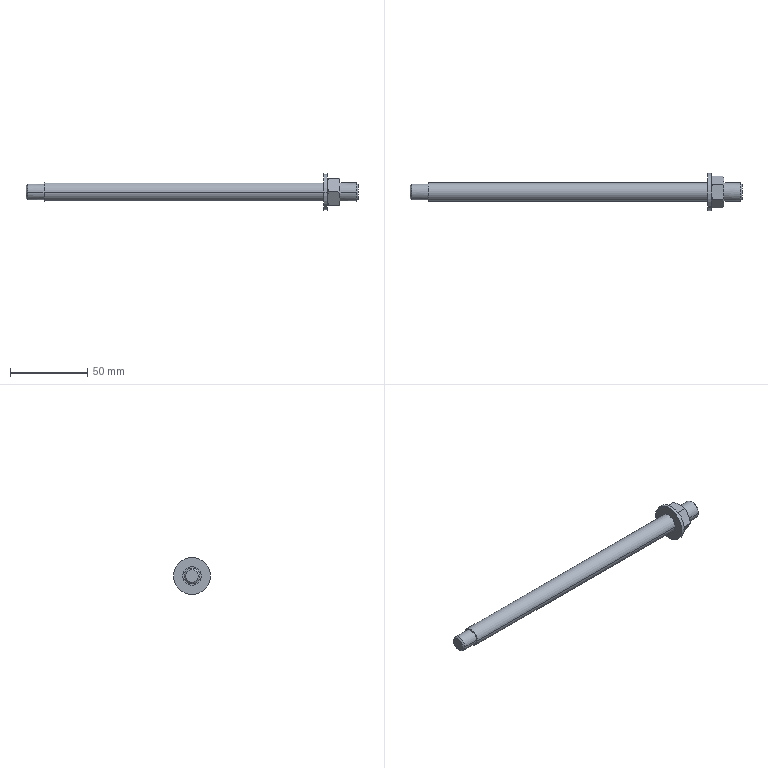Part | NX | features BREP 1 | 1 solid | 36 faces | box 215 x 24 x 24 mm | volume 26001 mm3 | cone 16 | plane 12 | cylinder 8 | commonest cylinder face diameters 12 x4 10.2 x2 24 x2
STEP:
#1=CARTESIAN_POINT('',(0.,-6.,0.));
#2=VERTEX_POINT('',#1);
#3=CARTESIAN_POINT('',(0.,6.,0.));
#4=VERTEX_POINT('',#3);
#5=CARTESIAN_POINT('',(0.,0.,0.));
#6=DIRECTION('',(-1.,0.,0.));
#7=DIRECTION('',(0.,-1.,0.));
#8=AXIS2_PLACEMENT_3D('',#5,#6,#7);
#9=CIRCLE('',#8,6.);
#10=EDGE_CURVE('',#2,#4,#9,.T.);
#11=ORIENTED_EDGE('',*,*,#10,.T.);
#12=CARTESIAN_POINT('',(-181.107,6.,0.));
#13=VERTEX_POINT('',#12);
#14=CARTESIAN_POINT('',(-192.773,6.,0.));
#15=DIRECTION('',(-1.,0.,0.));
#16=VECTOR('',#15,1000.);
#17=LINE('',#14,#16);
#18=EDGE_CURVE('',#4,#13,#17,.T.);
#19=ORIENTED_EDGE('',*,*,#18,.T.);
#20=CARTESIAN_POINT('',(-181.107,-6.,0.));
#21=VERTEX_POINT('',#20);
#22=CARTESIAN_POINT('',(-181.107,0.,0.));
#23=DIRECTION('',(1.,0.,0.));
#24=DIRECTION('',(0.,-1.,0.));
#25=AXIS2_PLACEMENT_3D('',#22,#23,#24);
#26=CIRCLE('',#25,6.);
#27=EDGE_CURVE('',#13,#21,#26,.T.);
#28=ORIENTED_EDGE('',*,*,#27,.T.);
#29=CARTESIAN_POINT('',(-192.773,-6.,0.));
#30=DIRECTION('',(-1.,0.,0.));
#31=VECTOR('',#30,1000.);
#32=LINE('',#29,#31);
#33=EDGE_CURVE('',#2,#21,#32,.T.);
#34=ORIENTED_EDGE('',*,*,#33,.F.);
#35=EDGE_LOOP('',(#11,#19,#28,#34));
#36=FACE_BOUND('',#35,.T.);
#37=CARTESIAN_POINT('',(-192.773,0.,0.));
#38=DIRECTION('',(-1.,0.,0.));
#39=DIRECTION('',(0.,-1.,0.));
#40=AXIS2_PLACEMENT_3D('',#37,#38,#39);
#41=CYLINDRICAL_SURFACE('',#40,6.);
#42=ADVANCED_FACE('',(#36),#41,.T.);
#43=CARTESIAN_POINT('',(-181.107,-5.1,0.));
#44=VERTEX_POINT('',#43);
#45=CARTESIAN_POINT('',(-181.107,5.1,0.));
#46=VERTEX_POINT('',#45);
#47=CARTESIAN_POINT('',(-181.107,0.,0.));
#48=DIRECTION('',(-1.,0.,0.));
#49=DIRECTION('',(0.,-1.,0.));
#50=AXIS2_PLACEMENT_3D('',#47,#48,#49);
#51=CIRCLE('',#50,5.1);
#52=EDGE_CURVE('',#44,#46,#51,.T.);
#53=ORIENTED_EDGE('',*,*,#52,.T.);
#54=CARTESIAN_POINT('',(-191.753,5.1,0.));
#55=VERTEX_POINT('',#54);
#56=CARTESIAN_POINT('',(-192.773,5.1,0.));
#57=DIRECTION('',(-1.,0.,0.));
#58=VECTOR('',#57,1000.);
#59=LINE('',#56,#58);
#60=EDGE_CURVE('',#46,#55,#59,.T.);
#61=ORIENTED_EDGE('',*,*,#60,.T.);
#62=CARTESIAN_POINT('',(-191.753,0.,5.1));
#63=VERTEX_POINT('',#62);
#64=CARTESIAN_POINT('',(-191.753,0.,0.));
#65=DIRECTION('',(1.,0.,0.));
#66=DIRECTION('',(0.,-1.,0.));
#67=AXIS2_PLACEMENT_3D('',#64,#65,#66);
#68=CIRCLE('',#67,5.1);
#69=EDGE_CURVE('',#55,#63,#68,.T.);
#70=ORIENTED_EDGE('',*,*,#69,.T.);
#71=CARTESIAN_POINT('',(-191.753,-5.1,0.));
#72=VERTEX_POINT('',#71);
#73=CARTESIAN_POINT('',(-191.753,0.,0.));
#74=DIRECTION('',(1.,0.,0.));
#75=DIRECTION('',(0.,-1.,0.));
#76=AXIS2_PLACEMENT_3D('',#73,#74,#75);
#77=CIRCLE('',#76,5.1);
#78=EDGE_CURVE('',#63,#72,#77,.T.);
#79=ORIENTED_EDGE('',*,*,#78,.T.);
#80=CARTESIAN_POINT('',(-192.773,-5.1,0.));
#81=DIRECTION('',(-1.,0.,0.));
#82=VECTOR('',#81,1000.);
#83=LINE('',#80,#82);
#84=EDGE_CURVE('',#44,#72,#83,.T.);
#85=ORIENTED_EDGE('',*,*,#84,.F.);
#86=EDGE_LOOP('',(#53,#61,#70,#79,#85));
#87=FACE_BOUND('',#86,.T.);
#88=CARTESIAN_POINT('',(-192.773,0.,0.));
#89=DIRECTION('',(-1.,0.,0.));
#90=DIRECTION('',(0.,-1.,0.));
#91=AXIS2_PLACEMENT_3D('',#88,#89,#90);
#92=CYLINDRICAL_SURFACE('',#91,5.1);
#93=ADVANCED_FACE('',(#87),#92,.T.);
#94=CARTESIAN_POINT('',(2.4,-12.,0.));
#95=VERTEX_POINT('',#94);
#96=CARTESIAN_POINT('',(2.4,12.,0.));
#97=VERTEX_POINT('',#96);
#98=CARTESIAN_POINT('',(2.4,0.,0.));
#99=DIRECTION('',(-1.,0.,0.));
#100=DIRECTION('',(0.,-1.,0.));
#101=AXIS2_PLACEMENT_3D('',#98,#99,#100);
#102=CIRCLE('',#101,12.);
#103=EDGE_CURVE('',#95,#97,#102,.T.);
#104=ORIENTED_EDGE('',*,*,#103,.T.);
#105=CARTESIAN_POINT('',(0.,12.,0.));
#106=VERTEX_POINT('',#105);
#107=CARTESIAN_POINT('',(-192.773,12.,0.));
#108=DIRECTION('',(-1.,0.,0.));
#109=VECTOR('',#108,1000.);
#110=LINE('',#107,#109);
#111=EDGE_CURVE('',#97,#106,#110,.T.);
#112=ORIENTED_EDGE('',*,*,#111,.T.);
#113=CARTESIAN_POINT('',(0.,-12.,0.));
#114=VERTEX_POINT('',#113);
#115=CARTESIAN_POINT('',(0.,0.,0.));
#116=DIRECTION('',(1.,0.,0.));
#117=DIRECTION('',(0.,-1.,0.));
#118=AXIS2_PLACEMENT_3D('',#115,#116,#117);
#119=CIRCLE('',#118,12.);
#120=EDGE_CURVE('',#106,#114,#119,.T.);
#121=ORIENTED_EDGE('',*,*,#120,.T.);
#122=CARTESIAN_POINT('',(-192.773,-12.,0.));
#123=DIRECTION('',(-1.,0.,0.));
#124=VECTOR('',#123,1000.);
#125=LINE('',#122,#124);
#126=EDGE_CURVE('',#95,#114,#125,.T.);
#127=ORIENTED_EDGE('',*,*,#126,.F.);
#128=EDGE_LOOP('',(#104,#112,#121,#127));
#129=FACE_BOUND('',#128,.T.);
#130=CARTESIAN_POINT('',(-192.773,0.,0.));
#131=DIRECTION('',(-1.,0.,0.));
#132=DIRECTION('',(0.,-1.,0.));
#133=AXIS2_PLACEMENT_3D('',#130,#131,#132);
#134=CYLINDRICAL_SURFACE('',#133,12.);
#135=ADVANCED_FACE('',(#129),#134,.T.);
#136=CARTESIAN_POINT('',(-192.773,0.,-4.08));
#137=VERTEX_POINT('',#136);
#138=CARTESIAN_POINT('',(-192.773,0.,4.08));
#139=VERTEX_POINT('',#138);
#140=CARTESIAN_POINT('',(-192.773,0.,0.));
#141=DIRECTION('',(1.,0.,0.));
#142=DIRECTION('',(0.,0.,-1.));
#143=AXIS2_PLACEMENT_3D('',#140,#141,#142);
#144=CIRCLE('',#143,4.08);
#145=EDGE_CURVE('',#137,#139,#144,.T.);
#146=ORIENTED_EDGE('',*,*,#145,.T.);
#147=CARTESIAN_POINT('',(-191.753,0.,5.1));
#148=DIRECTION('',(0.7071,0.,0.7071));
#149=VECTOR('',#148,1000.);
#150=LINE('',#147,#149);
#151=EDGE_CURVE('',#139,#63,#150,.T.);
#152=ORIENTED_EDGE('',*,*,#151,.T.);
#153=ORIENTED_EDGE('',*,*,#69,.F.);
#154=CARTESIAN_POINT('',(-191.753,0.,-5.1));
#155=VERTEX_POINT('',#154);
#156=CARTESIAN_POINT('',(-191.753,0.,0.));
#157=DIRECTION('',(1.,0.,0.));
#158=DIRECTION('',(0.,-1.,0.));
#159=AXIS2_PLACEMENT_3D('',#156,#157,#158);
#160=CIRCLE('',#159,5.1);
#161=EDGE_CURVE('',#155,#55,#160,.T.);
#162=ORIENTED_EDGE('',*,*,#161,.F.);
#163=CARTESIAN_POINT('',(-191.753,0.,-5.1));
#164=DIRECTION('',(0.7071,0.,-0.7071));
#165=VECTOR('',#164,1000.);
#166=LINE('',#163,#165);
#167=EDGE_CURVE('',#137,#155,#166,.T.);
#168=ORIENTED_EDGE('',*,*,#167,.F.);
#169=EDGE_LOOP('',(#146,#152,#153,#162,#168));
#170=FACE_BOUND('',#169,.T.);
#171=CARTESIAN_POINT('',(-191.753,0.,0.));
#172=DIRECTION('',(1.,0.,0.));
#173=DIRECTION('',(0.,0.,-1.));
#174=AXIS2_PLACEMENT_3D('',#171,#172,#173);
#175=CONICAL_SURFACE('',#174,5.1,0.7854);
#176=ADVANCED_FACE('',(#170),#175,.T.);
#177=CARTESIAN_POINT('',(21.207,0.,6.));
#178=VERTEX_POINT('',#177);
#179=CARTESIAN_POINT('',(21.207,6.,0.));
#180=VERTEX_POINT('',#179);
#181=CARTESIAN_POINT('',(21.207,0.,0.));
#182=DIRECTION('',(-1.,0.,0.));
#183=DIRECTION('',(0.,-1.,0.));
#184=AXIS2_PLACEMENT_3D('',#181,#182,#183);
#185=CIRCLE('',#184,6.);
#186=EDGE_CURVE('',#178,#180,#185,.T.);
#187=ORIENTED_EDGE('',*,*,#186,.T.);
#188=CARTESIAN_POINT('',(10.56,6.,0.));
#189=VERTEX_POINT('',#188);
#190=CARTESIAN_POINT('',(-192.773,6.,0.));
#191=DIRECTION('',(-1.,0.,0.));
#192=VECTOR('',#191,1000.);
#193=LINE('',#190,#192);
#194=EDGE_CURVE('',#180,#189,#193,.T.);
#195=ORIENTED_EDGE('',*,*,#194,.T.);
#196=CARTESIAN_POINT('',(10.56,-6.,0.));
#197=VERTEX_POINT('',#196);
#198=CARTESIAN_POINT('',(10.56,0.,0.));
#199=DIRECTION('',(1.,0.,0.));
#200=DIRECTION('',(0.,-1.,0.));
#201=AXIS2_PLACEMENT_3D('',#198,#199,#200);
#202=CIRCLE('',#201,6.);
#203=EDGE_CURVE('',#189,#197,#202,.T.);
#204=ORIENTED_EDGE('',*,*,#203,.T.);
#205=CARTESIAN_POINT('',(21.207,-6.,0.));
#206=VERTEX_POINT('',#205);
#207=CARTESIAN_POINT('',(-192.773,-6.,0.));
#208=DIRECTION('',(-1.,0.,0.));
#209=VECTOR('',#208,1000.);
#210=LINE('',#207,#209);
#211=EDGE_CURVE('',#206,#197,#210,.T.);
#212=ORIENTED_EDGE('',*,*,#211,.F.);
#213=CARTESIAN_POINT('',(21.207,0.,0.));
#214=DIRECTION('',(-1.,0.,0.));
#215=DIRECTION('',(0.,-1.,0.));
#216=AXIS2_PLACEMENT_3D('',#213,#214,#215);
#217=CIRCLE('',#216,6.);
#218=EDGE_CURVE('',#206,#178,#217,.T.);
#219=ORIENTED_EDGE('',*,*,#218,.T.);
#220=EDGE_LOOP('',(#187,#195,#204,#212,#219));
#221=FACE_BOUND('',#220,.T.);
#222=CARTESIAN_POINT('',(-192.773,0.,0.));
#223=DIRECTION('',(-1.,0.,0.));
#224=DIRECTION('',(0.,-1.,0.));
#225=AXIS2_PLACEMENT_3D('',#222,#223,#224);
#226=CYLINDRICAL_SURFACE('',#225,6.);
#227=ADVANCED_FACE('',(#221),#226,.T.);
#228=CARTESIAN_POINT('',(22.227,0.,4.98));
#229=VERTEX_POINT('',#228);
#230=CARTESIAN_POINT('',(22.227,0.,-4.98));
#231=VERTEX_POINT('',#230);
#232=CARTESIAN_POINT('',(22.227,0.,0.));
#233=DIRECTION('',(-1.,0.,0.));
#234=DIRECTION('',(0.,0.,1.));
#235=AXIS2_PLACEMENT_3D('',#232,#233,#234);
#236=CIRCLE('',#235,4.98);
#237=EDGE_CURVE('',#229,#231,#236,.T.);
#238=ORIENTED_EDGE('',*,*,#237,.T.);
#239=CARTESIAN_POINT('',(21.207,0.,-6.));
#240=VERTEX_POINT('',#239);
#241=CARTESIAN_POINT('',(21.207,0.,-6.));
#242=DIRECTION('',(-0.7071,0.,-0.7071));
#243=VECTOR('',#242,1000.);
#244=LINE('',#241,#243);
#245=EDGE_CURVE('',#240,#231,#244,.F.);
#246=ORIENTED_EDGE('',*,*,#245,.F.);
#247=CARTESIAN_POINT('',(21.207,0.,0.));
#248=DIRECTION('',(-1.,0.,0.));
#249=DIRECTION('',(0.,-1.,0.));
#250=AXIS2_PLACEMENT_3D('',#247,#248,#249);
#251=CIRCLE('',#250,6.);
#252=EDGE_CURVE('',#180,#240,#251,.T.);
#253=ORIENTED_EDGE('',*,*,#252,.F.);
#254=ORIENTED_EDGE('',*,*,#186,.F.);
#255=CARTESIAN_POINT('',(21.207,0.,6.));
#256=DIRECTION('',(-0.7071,0.,0.7071));
#257=VECTOR('',#256,1000.);
#258=LINE('',#255,#257);
#259=EDGE_CURVE('',#178,#229,#258,.F.);
#260=ORIENTED_EDGE('',*,*,#259,.T.);
#261=EDGE_LOOP('',(#238,#246,#253,#254,#260));
#262=FACE_BOUND('',#261,.T.);
#263=CARTESIAN_POINT('',(21.207,0.,0.));
#264=DIRECTION('',(-1.,0.,0.));
#265=DIRECTION('',(0.,0.,1.));
#266=AXIS2_PLACEMENT_3D('',#263,#264,#265);
#267=CONICAL_SURFACE('',#266,6.,0.7854);
#268=ADVANCED_FACE('',(#262),#267,.T.);
#269=ORIENTED_EDGE('',*,*,#18,.F.);
#270=CARTESIAN_POINT('',(0.,0.,0.));
#271=DIRECTION('',(-1.,0.,0.));
#272=DIRECTION('',(0.,-1.,0.));
#273=AXIS2_PLACEMENT_3D('',#270,#271,#272);
#274=CIRCLE('',#273,6.);
#275=EDGE_CURVE('',#4,#2,#274,.T.);
#276=ORIENTED_EDGE('',*,*,#275,.T.);
#277=ORIENTED_EDGE('',*,*,#33,.T.);
#278=CARTESIAN_POINT('',(-181.107,0.,0.));
#279=DIRECTION('',(1.,0.,0.));
#280=DIRECTION('',(0.,-1.,0.));
#281=AXIS2_PLACEMENT_3D('',#278,#279,#280);
#282=CIRCLE('',#281,6.);
#283=EDGE_CURVE('',#21,#13,#282,.T.);
#284=ORIENTED_EDGE('',*,*,#283,.T.);
#285=EDGE_LOOP('',(#269,#276,#277,#284));
#286=FACE_BOUND('',#285,.T.);
#287=CARTESIAN_POINT('',(-192.773,0.,0.));
#288=DIRECTION('',(-1.,0.,0.));
#289=DIRECTION('',(0.,-1.,0.));
#290=AXIS2_PLACEMENT_3D('',#287,#288,#289);
#291=CYLINDRICAL_SURFACE('',#290,6.);
#292=ADVANCED_FACE('',(#286),#291,.T.);
#293=ORIENTED_EDGE('',*,*,#283,.F.);
#294=ORIENTED_EDGE('',*,*,#27,.F.);
#295=EDGE_LOOP('',(#293,#294));
#296=FACE_BOUND('',#295,.T.);
#297=ORIENTED_EDGE('',*,*,#52,.F.);
#298=CARTESIAN_POINT('',(-181.107,0.,0.));
#299=DIRECTION('',(-1.,0.,0.));
#300=DIRECTION('',(0.,-1.,0.));
#301=AXIS2_PLACEMENT_3D('',#298,#299,#300);
#302=CIRCLE('',#301,5.1);
#303=EDGE_CURVE('',#46,#44,#302,.T.);
#304=ORIENTED_EDGE('',*,*,#303,.F.);
#305=EDGE_LOOP('',(#297,#304));
#306=FACE_BOUND('',#305,.T.);
#307=CARTESIAN_POINT('',(-181.107,5.1,0.));
#308=DIRECTION('',(1.,0.,0.));
#309=DIRECTION('',(0.,-1.,0.));
#310=AXIS2_PLACEMENT_3D('',#307,#308,#309);
#311=PLANE('',#310);
#312=ADVANCED_FACE('',(#296,#306),#311,.F.);
#313=CARTESIAN_POINT('',(0.,0.,0.));
#314=DIRECTION('',(1.,0.,0.));
#315=DIRECTION('',(0.,-1.,0.));
#316=AXIS2_PLACEMENT_3D('',#313,#314,#315);
#317=CIRCLE('',#316,12.);
#318=EDGE_CURVE('',#114,#106,#317,.T.);
#319=ORIENTED_EDGE('',*,*,#318,.F.);
#320=ORIENTED_EDGE('',*,*,#120,.F.);
#321=EDGE_LOOP('',(#319,#320));
#322=FACE_BOUND('',#321,.T.);
#323=ORIENTED_EDGE('',*,*,#10,.F.);
#324=ORIENTED_EDGE('',*,*,#275,.F.);
#325=EDGE_LOOP('',(#323,#324));
#326=FACE_BOUND('',#325,.T.);
#327=CARTESIAN_POINT('',(0.,6.,0.));
#328=DIRECTION('',(1.,0.,0.));
#329=DIRECTION('',(0.,-1.,0.));
#330=AXIS2_PLACEMENT_3D('',#327,#328,#329);
#331=PLANE('',#330);
#332=ADVANCED_FACE('',(#322,#326),#331,.F.);
#333=ORIENTED_EDGE('',*,*,#60,.F.);
#334=ORIENTED_EDGE('',*,*,#303,.T.);
#335=ORIENTED_EDGE('',*,*,#84,.T.);
#336=CARTESIAN_POINT('',(-191.753,0.,0.));
#337=DIRECTION('',(1.,0.,0.));
#338=DIRECTION('',(0.,-1.,0.));
#339=AXIS2_PLACEMENT_3D('',#336,#337,#338);
#340=CIRCLE('',#339,5.1);
#341=EDGE_CURVE('',#72,#155,#340,.T.);
#342=ORIENTED_EDGE('',*,*,#341,.T.);
#343=ORIENTED_EDGE('',*,*,#161,.T.);
#344=EDGE_LOOP('',(#333,#334,#335,#342,#343));
#345=FACE_BOUND('',#344,.T.);
#346=CARTESIAN_POINT('',(-192.773,0.,0.));
#347=DIRECTION('',(-1.,0.,0.));
#348=DIRECTION('',(0.,-1.,0.));
#349=AXIS2_PLACEMENT_3D('',#346,#347,#348);
#350=CYLINDRICAL_SURFACE('',#349,5.1);
#351=ADVANCED_FACE('',(#345),#350,.T.);
#352=ORIENTED_EDGE('',*,*,#111,.F.);
#353=CARTESIAN_POINT('',(2.4,0.,0.));
#354=DIRECTION('',(-1.,0.,0.));
#355=DIRECTION('',(0.,-1.,0.));
#356=AXIS2_PLACEMENT_3D('',#353,#354,#355);
#357=CIRCLE('',#356,12.);
#358=EDGE_CURVE('',#97,#95,#357,.T.);
#359=ORIENTED_EDGE('',*,*,#358,.T.);
#360=ORIENTED_EDGE('',*,*,#126,.T.);
#361=ORIENTED_EDGE('',*,*,#318,.T.);
#362=EDGE_LOOP('',(#352,#359,#360,#361));
#363=FACE_BOUND('',#362,.T.);
#364=CARTESIAN_POINT('',(-192.773,0.,0.));
#365=DIRECTION('',(-1.,0.,0.));
#366=DIRECTION('',(0.,-1.,0.));
#367=AXIS2_PLACEMENT_3D('',#364,#365,#366);
#368=CYLINDRICAL_SURFACE('',#367,12.);
#369=ADVANCED_FACE('',(#363),#368,.T.);
#370=ORIENTED_EDGE('',*,*,#151,.F.);
#371=CARTESIAN_POINT('',(-192.773,0.,0.));
#372=DIRECTION('',(1.,0.,0.));
#373=DIRECTION('',(0.,0.,-1.));
#374=AXIS2_PLACEMENT_3D('',#371,#372,#373);
#375=CIRCLE('',#374,4.08);
#376=EDGE_CURVE('',#139,#137,#375,.T.);
#377=ORIENTED_EDGE('',*,*,#376,.T.);
#378=ORIENTED_EDGE('',*,*,#167,.T.);
#379=ORIENTED_EDGE('',*,*,#341,.F.);
#380=ORIENTED_EDGE('',*,*,#78,.F.);
#381=EDGE_LOOP('',(#370,#377,#378,#379,#380));
#382=FACE_BOUND('',#381,.T.);
#383=CARTESIAN_POINT('',(-191.753,0.,0.));
#384=DIRECTION('',(1.,0.,0.));
#385=DIRECTION('',(0.,0.,-1.));
#386=AXIS2_PLACEMENT_3D('',#383,#384,#385);
#387=CONICAL_SURFACE('',#386,5.1,0.7854);
#388=ADVANCED_FACE('',(#382),#387,.T.);
#389=ORIENTED_EDGE('',*,*,#103,.F.);
#390=ORIENTED_EDGE('',*,*,#358,.F.);
#391=EDGE_LOOP('',(#389,#390));
#392=FACE_BOUND('',#391,.T.);
#393=CARTESIAN_POINT('',(2.4,7.65,-4.417));
#394=VERTEX_POINT('',#393);
#395=CARTESIAN_POINT('',(2.4,7.65,4.417));
#396=VERTEX_POINT('',#395);
#397=CARTESIAN_POINT('',(2.4,0.,0.));
#398=DIRECTION('',(1.,0.,0.));
#399=DIRECTION('',(0.,0.,-1.));
#400=AXIS2_PLACEMENT_3D('',#397,#398,#399);
#401=CIRCLE('',#400,8.833);
#402=EDGE_CURVE('',#394,#396,#401,.T.);
#403=ORIENTED_EDGE('',*,*,#402,.F.);
#404=CARTESIAN_POINT('',(2.4,0.,-8.833));
#405=VERTEX_POINT('',#404);
#406=CARTESIAN_POINT('',(2.4,0.,0.));
#407=DIRECTION('',(1.,0.,0.));
#408=DIRECTION('',(0.,0.,-1.));
#409=AXIS2_PLACEMENT_3D('',#406,#407,#408);
#410=CIRCLE('',#409,8.833);
#411=EDGE_CURVE('',#405,#394,#410,.T.);
#412=ORIENTED_EDGE('',*,*,#411,.F.);
#413=CARTESIAN_POINT('',(2.4,-7.65,-4.417));
#414=VERTEX_POINT('',#413);
#415=CARTESIAN_POINT('',(2.4,0.,0.));
#416=DIRECTION('',(1.,0.,0.));
#417=DIRECTION('',(0.,0.,-1.));
#418=AXIS2_PLACEMENT_3D('',#415,#416,#417);
#419=CIRCLE('',#418,8.833);
#420=EDGE_CURVE('',#414,#405,#419,.T.);
#421=ORIENTED_EDGE('',*,*,#420,.F.);
#422=CARTESIAN_POINT('',(2.4,-7.65,4.417));
#423=VERTEX_POINT('',#422);
#424=CARTESIAN_POINT('',(2.4,0.,0.));
#425=DIRECTION('',(1.,0.,0.));
#426=DIRECTION('',(0.,0.,-1.));
#427=AXIS2_PLACEMENT_3D('',#424,#425,#426);
#428=CIRCLE('',#427,8.833);
#429=EDGE_CURVE('',#423,#414,#428,.T.);
#430=ORIENTED_EDGE('',*,*,#429,.F.);
#431=CARTESIAN_POINT('',(2.4,0.,8.833));
#432=VERTEX_POINT('',#431);
#433=CARTESIAN_POINT('',(2.4,0.,0.));
#434=DIRECTION('',(1.,0.,0.));
#435=DIRECTION('',(0.,0.,-1.));
#436=AXIS2_PLACEMENT_3D('',#433,#434,#435);
#437=CIRCLE('',#436,8.833);
#438=EDGE_CURVE('',#432,#423,#437,.T.);
#439=ORIENTED_EDGE('',*,*,#438,.F.);
#440=CARTESIAN_POINT('',(2.4,0.,0.));
#441=DIRECTION('',(1.,0.,0.));
#442=DIRECTION('',(0.,0.,-1.));
#443=AXIS2_PLACEMENT_3D('',#440,#441,#442);
#444=CIRCLE('',#443,8.833);
#445=EDGE_CURVE('',#396,#432,#444,.T.);
#446=ORIENTED_EDGE('',*,*,#445,.F.);
#447=EDGE_LOOP('',(#403,#412,#421,#430,#439,#446));
#448=FACE_BOUND('',#447,.T.);
#449=CARTESIAN_POINT('',(2.4,12.,0.));
#450=DIRECTION('',(-1.,0.,0.));
#451=DIRECTION('',(0.,0.,1.));
#452=AXIS2_PLACEMENT_3D('',#449,#450,#451);
#453=PLANE('',#452);
#454=ADVANCED_FACE('',(#392,#448),#453,.F.);
#455=ORIENTED_EDGE('',*,*,#145,.F.);
#456=ORIENTED_EDGE('',*,*,#376,.F.);
#457=EDGE_LOOP('',(#455,#456));
#458=FACE_BOUND('',#457,.T.);
#459=CARTESIAN_POINT('',(-192.773,0.,0.));
#460=DIRECTION('',(1.,0.,0.));
#461=DIRECTION('',(0.,-1.,0.));
#462=AXIS2_PLACEMENT_3D('',#459,#460,#461);
#463=PLANE('',#462);
#464=ADVANCED_FACE('',(#458),#463,.F.);
#465=ORIENTED_EDGE('',*,*,#402,.T.);
#466=CARTESIAN_POINT('',(3.189,10.2,0.));
#467=VERTEX_POINT('',#466);
#468=CARTESIAN_POINT('',(3.189,10.2,0.));
#469=CARTESIAN_POINT('',(2.934,9.758,0.7653));
#470=CARTESIAN_POINT('',(2.559,8.964,2.142));
#471=CARTESIAN_POINT('',(2.4,8.071,3.688));
#472=CARTESIAN_POINT('',(2.4,7.65,4.417));
#473=B_SPLINE_CURVE_WITH_KNOTS('',3,(#468,#469,#470,#471,#472),.UNSPECIFIED.,.F.,.F.,(4,1,4),(0.,0.5,1.),.UNSPECIFIED.);
#474=EDGE_CURVE('',#396,#467,#473,.F.);
#475=ORIENTED_EDGE('',*,*,#474,.T.);
#476=CARTESIAN_POINT('',(2.4,7.65,-4.417));
#477=CARTESIAN_POINT('',(2.4,8.071,-3.688));
#478=CARTESIAN_POINT('',(2.559,8.964,-2.141));
#479=CARTESIAN_POINT('',(2.934,9.758,-0.7656));
#480=CARTESIAN_POINT('',(3.189,10.2,0.));
#481=B_SPLINE_CURVE_WITH_KNOTS('',3,(#476,#477,#478,#479,#480),.UNSPECIFIED.,.F.,.F.,(4,1,4),(0.,0.5,1.),.UNSPECIFIED.);
#482=EDGE_CURVE('',#467,#394,#481,.F.);
#483=ORIENTED_EDGE('',*,*,#482,.T.);
#484=EDGE_LOOP('',(#465,#475,#483));
#485=FACE_BOUND('',#484,.T.);
#486=CARTESIAN_POINT('',(3.194,0.,0.));
#487=DIRECTION('',(1.,0.,0.));
#488=DIRECTION('',(0.,0.,-1.));
#489=AXIS2_PLACEMENT_3D('',#486,#487,#488);
#490=CONICAL_SURFACE('',#489,10.208,1.047);
#491=ADVANCED_FACE('',(#485),#490,.T.);
#492=CARTESIAN_POINT('',(3.189,5.1,-8.833));
#493=VERTEX_POINT('',#492);
#494=CARTESIAN_POINT('',(3.189,5.1,-8.833));
#495=CARTESIAN_POINT('',(2.934,5.542,-8.068));
#496=CARTESIAN_POINT('',(2.559,6.336,-6.692));
#497=CARTESIAN_POINT('',(2.4,7.229,-5.146));
#498=CARTESIAN_POINT('',(2.4,7.65,-4.417));
#499=B_SPLINE_CURVE_WITH_KNOTS('',3,(#494,#495,#496,#497,#498),.UNSPECIFIED.,.F.,.F.,(4,1,4),(0.,0.5,1.),.UNSPECIFIED.);
#500=EDGE_CURVE('',#394,#493,#499,.F.);
#501=ORIENTED_EDGE('',*,*,#500,.T.);
#502=CARTESIAN_POINT('',(2.4,0.,-8.833));
#503=CARTESIAN_POINT('',(2.4,0.8417,-8.833));
#504=CARTESIAN_POINT('',(2.559,2.627,-8.833));
#505=CARTESIAN_POINT('',(2.934,4.216,-8.833));
#506=CARTESIAN_POINT('',(3.189,5.1,-8.833));
#507=B_SPLINE_CURVE_WITH_KNOTS('',3,(#502,#503,#504,#505,#506),.UNSPECIFIED.,.F.,.F.,(4,1,4),(0.,0.5,1.),.UNSPECIFIED.);
#508=EDGE_CURVE('',#493,#405,#507,.F.);
#509=ORIENTED_EDGE('',*,*,#508,.T.);
#510=ORIENTED_EDGE('',*,*,#411,.T.);
#511=EDGE_LOOP('',(#501,#509,#510));
#512=FACE_BOUND('',#511,.T.);
#513=CARTESIAN_POINT('',(3.194,0.,0.));
#514=DIRECTION('',(1.,0.,0.));
#515=DIRECTION('',(0.,0.,-1.));
#516=AXIS2_PLACEMENT_3D('',#513,#514,#515);
#517=CONICAL_SURFACE('',#516,10.208,1.047);
#518=ADVANCED_FACE('',(#512),#517,.T.);
#519=CARTESIAN_POINT('',(3.189,-5.1,-8.833));
#520=VERTEX_POINT('',#519);
#521=CARTESIAN_POINT('',(3.189,-5.1,-8.833));
#522=CARTESIAN_POINT('',(2.934,-4.216,-8.833));
#523=CARTESIAN_POINT('',(2.559,-2.627,-8.833));
#524=CARTESIAN_POINT('',(2.4,-0.8419,-8.833));
#525=CARTESIAN_POINT('',(2.4,0.,-8.833));
#526=B_SPLINE_CURVE_WITH_KNOTS('',3,(#521,#522,#523,#524,#525),.UNSPECIFIED.,.F.,.F.,(4,1,4),(0.,0.5,1.),.UNSPECIFIED.);
#527=EDGE_CURVE('',#405,#520,#526,.F.);
#528=ORIENTED_EDGE('',*,*,#527,.T.);
#529=CARTESIAN_POINT('',(2.4,-7.65,-4.417));
#530=CARTESIAN_POINT('',(2.4,-7.229,-5.146));
#531=CARTESIAN_POINT('',(2.559,-6.336,-6.692));
#532=CARTESIAN_POINT('',(2.934,-5.542,-8.068));
#533=CARTESIAN_POINT('',(3.189,-5.1,-8.833));
#534=B_SPLINE_CURVE_WITH_KNOTS('',3,(#529,#530,#531,#532,#533),.UNSPECIFIED.,.F.,.F.,(4,1,4),(0.,0.5,1.),.UNSPECIFIED.);
#535=EDGE_CURVE('',#520,#414,#534,.F.);
#536=ORIENTED_EDGE('',*,*,#535,.T.);
#537=ORIENTED_EDGE('',*,*,#420,.T.);
#538=EDGE_LOOP('',(#528,#536,#537));
#539=FACE_BOUND('',#538,.T.);
#540=CARTESIAN_POINT('',(3.194,0.,0.));
#541=DIRECTION('',(1.,0.,0.));
#542=DIRECTION('',(0.,0.,-1.));
#543=AXIS2_PLACEMENT_3D('',#540,#541,#542);
#544=CONICAL_SURFACE('',#543,10.208,1.047);
#545=ADVANCED_FACE('',(#539),#544,.T.);
#546=ORIENTED_EDGE('',*,*,#429,.T.);
#547=CARTESIAN_POINT('',(3.189,-10.2,0.000000043));
#548=VERTEX_POINT('',#547);
#549=CARTESIAN_POINT('',(3.189,-10.2,0.000000022));
#550=CARTESIAN_POINT('',(2.934,-9.758,-0.7653));
#551=CARTESIAN_POINT('',(2.559,-8.964,-2.142));
#552=CARTESIAN_POINT('',(2.4,-8.071,-3.688));
#553=CARTESIAN_POINT('',(2.4,-7.65,-4.417));
#554=B_SPLINE_CURVE_WITH_KNOTS('',3,(#549,#550,#551,#552,#553),.UNSPECIFIED.,.F.,.F.,(4,1,4),(0.,0.5,1.),.UNSPECIFIED.);
#555=EDGE_CURVE('',#414,#548,#554,.F.);
#556=ORIENTED_EDGE('',*,*,#555,.T.);
#557=CARTESIAN_POINT('',(2.4,-7.65,4.417));
#558=CARTESIAN_POINT('',(2.4,-8.071,3.688));
#559=CARTESIAN_POINT('',(2.559,-8.964,2.141));
#560=CARTESIAN_POINT('',(2.934,-9.758,0.7656));
#561=CARTESIAN_POINT('',(3.189,-10.2,0.000000043));
#562=B_SPLINE_CURVE_WITH_KNOTS('',3,(#557,#558,#559,#560,#561),.UNSPECIFIED.,.F.,.F.,(4,1,4),(0.,0.5,1.),.UNSPECIFIED.);
#563=EDGE_CURVE('',#548,#423,#562,.F.);
#564=ORIENTED_EDGE('',*,*,#563,.T.);
#565=EDGE_LOOP('',(#546,#556,#564));
#566=FACE_BOUND('',#565,.T.);
#567=CARTESIAN_POINT('',(3.194,0.,0.));
#568=DIRECTION('',(1.,0.,0.));
#569=DIRECTION('',(0.,0.,-1.));
#570=AXIS2_PLACEMENT_3D('',#567,#568,#569);
#571=CONICAL_SURFACE('',#570,10.208,1.047);
#572=ADVANCED_FACE('',(#566),#571,.T.);
#573=ORIENTED_EDGE('',*,*,#438,.T.);
#574=CARTESIAN_POINT('',(3.189,-5.1,8.833));
#575=VERTEX_POINT('',#574);
#576=CARTESIAN_POINT('',(3.189,-5.1,8.833));
#577=CARTESIAN_POINT('',(2.934,-5.542,8.068));
#578=CARTESIAN_POINT('',(2.559,-6.336,6.692));
#579=CARTESIAN_POINT('',(2.4,-7.229,5.146));
#580=CARTESIAN_POINT('',(2.4,-7.65,4.417));
#581=B_SPLINE_CURVE_WITH_KNOTS('',3,(#576,#577,#578,#579,#580),.UNSPECIFIED.,.F.,.F.,(4,1,4),(0.,0.5,1.),.UNSPECIFIED.);
#582=EDGE_CURVE('',#423,#575,#581,.F.);
#583=ORIENTED_EDGE('',*,*,#582,.T.);
#584=CARTESIAN_POINT('',(2.4,0.,8.833));
#585=CARTESIAN_POINT('',(2.4,-0.8417,8.833));
#586=CARTESIAN_POINT('',(2.559,-2.627,8.833));
#587=CARTESIAN_POINT('',(2.934,-4.216,8.833));
#588=CARTESIAN_POINT('',(3.189,-5.1,8.833));
#589=B_SPLINE_CURVE_WITH_KNOTS('',3,(#584,#585,#586,#587,#588),.UNSPECIFIED.,.F.,.F.,(4,1,4),(0.,0.5,1.),.UNSPECIFIED.);
#590=EDGE_CURVE('',#575,#432,#589,.F.);
#591=ORIENTED_EDGE('',*,*,#590,.T.);
#592=EDGE_LOOP('',(#573,#583,#591));
#593=FACE_BOUND('',#592,.T.);
#594=CARTESIAN_POINT('',(3.194,0.,0.));
#595=DIRECTION('',(1.,0.,0.));
#596=DIRECTION('',(0.,0.,-1.));
#597=AXIS2_PLACEMENT_3D('',#594,#595,#596);
#598=CONICAL_SURFACE('',#597,10.208,1.047);
#599=ADVANCED_FACE('',(#593),#598,.T.);
#600=ORIENTED_EDGE('',*,*,#445,.T.);
#601=CARTESIAN_POINT('',(3.189,5.1,8.833));
#602=VERTEX_POINT('',#601);
#603=CARTESIAN_POINT('',(3.189,5.1,8.833));
#604=CARTESIAN_POINT('',(2.934,4.216,8.833));
#605=CARTESIAN_POINT('',(2.559,2.627,8.833));
#606=CARTESIAN_POINT('',(2.4,0.8419,8.833));
#607=CARTESIAN_POINT('',(2.4,0.,8.833));
#608=B_SPLINE_CURVE_WITH_KNOTS('',3,(#603,#604,#605,#606,#607),.UNSPECIFIED.,.F.,.F.,(4,1,4),(0.,0.5,1.),.UNSPECIFIED.);
#609=EDGE_CURVE('',#432,#602,#608,.F.);
#610=ORIENTED_EDGE('',*,*,#609,.T.);
#611=CARTESIAN_POINT('',(2.4,7.65,4.417));
#612=CARTESIAN_POINT('',(2.4,7.229,5.146));
#613=CARTESIAN_POINT('',(2.559,6.336,6.692));
#614=CARTESIAN_POINT('',(2.934,5.542,8.068));
#615=CARTESIAN_POINT('',(3.189,5.1,8.833));
#616=B_SPLINE_CURVE_WITH_KNOTS('',3,(#611,#612,#613,#614,#615),.UNSPECIFIED.,.F.,.F.,(4,1,4),(0.,0.5,1.),.UNSPECIFIED.);
#617=EDGE_CURVE('',#602,#396,#616,.F.);
#618=ORIENTED_EDGE('',*,*,#617,.T.);
#619=EDGE_LOOP('',(#600,#610,#618));
#620=FACE_BOUND('',#619,.T.);
#621=CARTESIAN_POINT('',(3.194,0.,0.));
#622=DIRECTION('',(1.,0.,0.));
#623=DIRECTION('',(0.,0.,-1.));
#624=AXIS2_PLACEMENT_3D('',#621,#622,#623);
#625=CONICAL_SURFACE('',#624,10.208,1.047);
#626=ADVANCED_FACE('',(#620),#625,.T.);
#627=CARTESIAN_POINT('',(9.771,5.1,8.833));
#628=VERTEX_POINT('',#627);
#629=CARTESIAN_POINT('',(10.56,7.65,4.417));
#630=VERTEX_POINT('',#629);
#631=CARTESIAN_POINT('',(9.771,5.1,8.833));
#632=CARTESIAN_POINT('',(10.026,5.542,8.068));
#633=CARTESIAN_POINT('',(10.401,6.337,6.692));
#634=CARTESIAN_POINT('',(10.56,7.229,5.146));
#635=CARTESIAN_POINT('',(10.56,7.65,4.417));
#636=B_SPLINE_CURVE_WITH_KNOTS('',3,(#631,#632,#633,#634,#635),.UNSPECIFIED.,.F.,.F.,(4,1,4),(0.,0.5,1.),.UNSPECIFIED.);
#637=EDGE_CURVE('',#628,#630,#636,.T.);
#638=ORIENTED_EDGE('',*,*,#637,.T.);
#639=CARTESIAN_POINT('',(9.771,10.2,0.));
#640=VERTEX_POINT('',#639);
#641=CARTESIAN_POINT('',(10.56,7.65,4.417));
#642=CARTESIAN_POINT('',(10.56,8.071,3.688));
#643=CARTESIAN_POINT('',(10.401,8.964,2.141));
#644=CARTESIAN_POINT('',(10.026,9.758,0.7658));
#645=CARTESIAN_POINT('',(9.771,10.2,0.));
#646=B_SPLINE_CURVE_WITH_KNOTS('',3,(#641,#642,#643,#644,#645),.UNSPECIFIED.,.F.,.F.,(4,1,4),(0.,0.5,1.),.UNSPECIFIED.);
#647=EDGE_CURVE('',#630,#640,#646,.T.);
#648=ORIENTED_EDGE('',*,*,#647,.T.);
#649=CARTESIAN_POINT('',(2.4,10.2,0.));
#650=DIRECTION('',(-1.,0.,0.));
#651=VECTOR('',#650,1000.);
#652=LINE('',#649,#651);
#653=EDGE_CURVE('',#640,#467,#652,.T.);
#654=ORIENTED_EDGE('',*,*,#653,.T.);
#655=ORIENTED_EDGE('',*,*,#474,.F.);
#656=ORIENTED_EDGE('',*,*,#617,.F.);
#657=CARTESIAN_POINT('',(2.4,5.1,8.833));
#658=DIRECTION('',(1.,0.,0.));
#659=VECTOR('',#658,1000.);
#660=LINE('',#657,#659);
#661=EDGE_CURVE('',#602,#628,#660,.T.);
#662=ORIENTED_EDGE('',*,*,#661,.T.);
#663=EDGE_LOOP('',(#638,#648,#654,#655,#656,#662));
#664=FACE_BOUND('',#663,.T.);
#665=CARTESIAN_POINT('',(2.4,10.2,0.));
#666=DIRECTION('',(0.,0.866,0.5));
#667=DIRECTION('',(1.,0.,0.));
#668=AXIS2_PLACEMENT_3D('',#665,#666,#667);
#669=PLANE('',#668);
#670=ADVANCED_FACE('',(#664),#669,.T.);
#671=CARTESIAN_POINT('',(10.56,7.65,-4.417));
#672=VERTEX_POINT('',#671);
#673=CARTESIAN_POINT('',(9.771,10.2,0.));
#674=CARTESIAN_POINT('',(10.026,9.758,-0.7651));
#675=CARTESIAN_POINT('',(10.401,8.963,-2.142));
#676=CARTESIAN_POINT('',(10.56,8.071,-3.687));
#677=CARTESIAN_POINT('',(10.56,7.65,-4.417));
#678=B_SPLINE_CURVE_WITH_KNOTS('',3,(#673,#674,#675,#676,#677),.UNSPECIFIED.,.F.,.F.,(4,1,4),(0.,0.5,1.),.UNSPECIFIED.);
#679=EDGE_CURVE('',#640,#672,#678,.T.);
#680=ORIENTED_EDGE('',*,*,#679,.T.);
#681=CARTESIAN_POINT('',(9.771,5.1,-8.833));
#682=VERTEX_POINT('',#681);
#683=CARTESIAN_POINT('',(10.56,7.65,-4.417));
#684=CARTESIAN_POINT('',(10.56,7.229,-5.145));
#685=CARTESIAN_POINT('',(10.401,6.336,-6.692));
#686=CARTESIAN_POINT('',(10.026,5.542,-8.068));
#687=CARTESIAN_POINT('',(9.771,5.1,-8.833));
#688=B_SPLINE_CURVE_WITH_KNOTS('',3,(#683,#684,#685,#686,#687),.UNSPECIFIED.,.F.,.F.,(4,1,4),(0.,0.5,1.),.UNSPECIFIED.);
#689=EDGE_CURVE('',#672,#682,#688,.T.);
#690=ORIENTED_EDGE('',*,*,#689,.T.);
#691=CARTESIAN_POINT('',(2.4,5.1,-8.833));
#692=DIRECTION('',(-1.,0.,0.));
#693=VECTOR('',#692,1000.);
#694=LINE('',#691,#693);
#695=EDGE_CURVE('',#682,#493,#694,.T.);
#696=ORIENTED_EDGE('',*,*,#695,.T.);
#697=ORIENTED_EDGE('',*,*,#500,.F.);
#698=ORIENTED_EDGE('',*,*,#482,.F.);
#699=ORIENTED_EDGE('',*,*,#653,.F.);
#700=EDGE_LOOP('',(#680,#690,#696,#697,#698,#699));
#701=FACE_BOUND('',#700,.T.);
#702=CARTESIAN_POINT('',(2.4,5.1,-8.833));
#703=DIRECTION('',(0.,0.866,-0.5));
#704=DIRECTION('',(-1.,0.,0.));
#705=AXIS2_PLACEMENT_3D('',#702,#703,#704);
#706=PLANE('',#705);
#707=ADVANCED_FACE('',(#701),#706,.T.);
#708=CARTESIAN_POINT('',(10.56,0.,-8.833));
#709=VERTEX_POINT('',#708);
#710=CARTESIAN_POINT('',(9.771,5.1,-8.833));
#711=CARTESIAN_POINT('',(10.026,4.216,-8.833));
#712=CARTESIAN_POINT('',(10.401,2.627,-8.833));
#713=CARTESIAN_POINT('',(10.56,0.8421,-8.833));
#714=CARTESIAN_POINT('',(10.56,0.,-8.833));
#715=B_SPLINE_CURVE_WITH_KNOTS('',3,(#710,#711,#712,#713,#714),.UNSPECIFIED.,.F.,.F.,(4,1,4),(0.,0.5,1.),.UNSPECIFIED.);
#716=EDGE_CURVE('',#682,#709,#715,.T.);
#717=ORIENTED_EDGE('',*,*,#716,.T.);
#718=CARTESIAN_POINT('',(9.771,-5.1,-8.833));
#719=VERTEX_POINT('',#718);
#720=CARTESIAN_POINT('',(10.56,0.,-8.833));
#721=CARTESIAN_POINT('',(10.56,-0.8414,-8.833));
#722=CARTESIAN_POINT('',(10.401,-2.628,-8.833));
#723=CARTESIAN_POINT('',(10.026,-4.216,-8.833));
#724=CARTESIAN_POINT('',(9.771,-5.1,-8.833));
#725=B_SPLINE_CURVE_WITH_KNOTS('',3,(#720,#721,#722,#723,#724),.UNSPECIFIED.,.F.,.F.,(4,1,4),(0.,0.5,1.),.UNSPECIFIED.);
#726=EDGE_CURVE('',#709,#719,#725,.T.);
#727=ORIENTED_EDGE('',*,*,#726,.T.);
#728=CARTESIAN_POINT('',(2.4,-5.1,-8.833));
#729=DIRECTION('',(-1.,0.,0.));
#730=VECTOR('',#729,1000.);
#731=LINE('',#728,#730);
#732=EDGE_CURVE('',#719,#520,#731,.T.);
#733=ORIENTED_EDGE('',*,*,#732,.T.);
#734=ORIENTED_EDGE('',*,*,#527,.F.);
#735=ORIENTED_EDGE('',*,*,#508,.F.);
#736=ORIENTED_EDGE('',*,*,#695,.F.);
#737=EDGE_LOOP('',(#717,#727,#733,#734,#735,#736));
#738=FACE_BOUND('',#737,.T.);
#739=CARTESIAN_POINT('',(2.4,-5.1,-8.833));
#740=DIRECTION('',(0.,0.,-1.));
#741=DIRECTION('',(-1.,0.,0.));
#742=AXIS2_PLACEMENT_3D('',#739,#740,#741);
#743=PLANE('',#742);
#744=ADVANCED_FACE('',(#738),#743,.T.);
#745=CARTESIAN_POINT('',(10.56,-7.65,-4.417));
#746=VERTEX_POINT('',#745);
#747=CARTESIAN_POINT('',(9.771,-5.1,-8.833));
#748=CARTESIAN_POINT('',(10.026,-5.542,-8.068));
#749=CARTESIAN_POINT('',(10.401,-6.337,-6.692));
#750=CARTESIAN_POINT('',(10.56,-7.229,-5.146));
#751=CARTESIAN_POINT('',(10.56,-7.65,-4.417));
#752=B_SPLINE_CURVE_WITH_KNOTS('',3,(#747,#748,#749,#750,#751),.UNSPECIFIED.,.F.,.F.,(4,1,4),(0.,0.5,1.),.UNSPECIFIED.);
#753=EDGE_CURVE('',#719,#746,#752,.T.);
#754=ORIENTED_EDGE('',*,*,#753,.T.);
#755=CARTESIAN_POINT('',(9.771,-10.2,0.));
#756=VERTEX_POINT('',#755);
#757=CARTESIAN_POINT('',(10.56,-7.65,-4.417));
#758=CARTESIAN_POINT('',(10.56,-8.071,-3.688));
#759=CARTESIAN_POINT('',(10.401,-8.964,-2.141));
#760=CARTESIAN_POINT('',(10.026,-9.758,-0.7658));
#761=CARTESIAN_POINT('',(9.771,-10.2,0.));
#762=B_SPLINE_CURVE_WITH_KNOTS('',3,(#757,#758,#759,#760,#761),.UNSPECIFIED.,.F.,.F.,(4,1,4),(0.,0.5,1.),.UNSPECIFIED.);
#763=EDGE_CURVE('',#746,#756,#762,.T.);
#764=ORIENTED_EDGE('',*,*,#763,.T.);
#765=CARTESIAN_POINT('',(2.4,-10.2,0.));
#766=DIRECTION('',(-1.,0.,0.));
#767=VECTOR('',#766,1000.);
#768=LINE('',#765,#767);
#769=EDGE_CURVE('',#756,#548,#768,.T.);
#770=ORIENTED_EDGE('',*,*,#769,.T.);
#771=ORIENTED_EDGE('',*,*,#555,.F.);
#772=ORIENTED_EDGE('',*,*,#535,.F.);
#773=ORIENTED_EDGE('',*,*,#732,.F.);
#774=EDGE_LOOP('',(#754,#764,#770,#771,#772,#773));
#775=FACE_BOUND('',#774,.T.);
#776=CARTESIAN_POINT('',(2.4,-10.2,0.));
#777=DIRECTION('',(0.,-0.866,-0.5));
#778=DIRECTION('',(0.,0.5,-0.866));
#779=AXIS2_PLACEMENT_3D('',#776,#777,#778);
#780=PLANE('',#779);
#781=ADVANCED_FACE('',(#775),#780,.T.);
#782=CARTESIAN_POINT('',(10.56,-7.65,4.417));
#783=VERTEX_POINT('',#782);
#784=CARTESIAN_POINT('',(9.771,-10.2,0.));
#785=CARTESIAN_POINT('',(10.026,-9.758,0.7651));
#786=CARTESIAN_POINT('',(10.401,-8.963,2.142));
#787=CARTESIAN_POINT('',(10.56,-8.071,3.687));
#788=CARTESIAN_POINT('',(10.56,-7.65,4.417));
#789=B_SPLINE_CURVE_WITH_KNOTS('',3,(#784,#785,#786,#787,#788),.UNSPECIFIED.,.F.,.F.,(4,1,4),(0.,0.5,1.),.UNSPECIFIED.);
#790=EDGE_CURVE('',#756,#783,#789,.T.);
#791=ORIENTED_EDGE('',*,*,#790,.T.);
#792=CARTESIAN_POINT('',(9.771,-5.1,8.833));
#793=VERTEX_POINT('',#792);
#794=CARTESIAN_POINT('',(10.56,-7.65,4.417));
#795=CARTESIAN_POINT('',(10.56,-7.229,5.145));
#796=CARTESIAN_POINT('',(10.401,-6.336,6.692));
#797=CARTESIAN_POINT('',(10.026,-5.542,8.068));
#798=CARTESIAN_POINT('',(9.771,-5.1,8.833));
#799=B_SPLINE_CURVE_WITH_KNOTS('',3,(#794,#795,#796,#797,#798),.UNSPECIFIED.,.F.,.F.,(4,1,4),(0.,0.5,1.),.UNSPECIFIED.);
#800=EDGE_CURVE('',#783,#793,#799,.T.);
#801=ORIENTED_EDGE('',*,*,#800,.T.);
#802=CARTESIAN_POINT('',(2.4,-5.1,8.833));
#803=DIRECTION('',(-1.,0.,0.));
#804=VECTOR('',#803,1000.);
#805=LINE('',#802,#804);
#806=EDGE_CURVE('',#793,#575,#805,.T.);
#807=ORIENTED_EDGE('',*,*,#806,.T.);
#808=ORIENTED_EDGE('',*,*,#582,.F.);
#809=ORIENTED_EDGE('',*,*,#563,.F.);
#810=ORIENTED_EDGE('',*,*,#769,.F.);
#811=EDGE_LOOP('',(#791,#801,#807,#808,#809,#810));
#812=FACE_BOUND('',#811,.T.);
#813=CARTESIAN_POINT('',(2.4,-5.1,8.833));
#814=DIRECTION('',(0.,-0.866,0.5));
#815=DIRECTION('',(-1.,0.,0.));
#816=AXIS2_PLACEMENT_3D('',#813,#814,#815);
#817=PLANE('',#816);
#818=ADVANCED_FACE('',(#812),#817,.T.);
#819=CARTESIAN_POINT('',(10.56,0.,8.833));
#820=VERTEX_POINT('',#819);
#821=CARTESIAN_POINT('',(9.771,-5.1,8.833));
#822=CARTESIAN_POINT('',(10.026,-4.216,8.833));
#823=CARTESIAN_POINT('',(10.401,-2.627,8.833));
#824=CARTESIAN_POINT('',(10.56,-0.8421,8.833));
#825=CARTESIAN_POINT('',(10.56,0.,8.833));
#826=B_SPLINE_CURVE_WITH_KNOTS('',3,(#821,#822,#823,#824,#825),.UNSPECIFIED.,.F.,.F.,(4,1,4),(0.,0.5,1.),.UNSPECIFIED.);
#827=EDGE_CURVE('',#793,#820,#826,.T.);
#828=ORIENTED_EDGE('',*,*,#827,.T.);
#829=CARTESIAN_POINT('',(10.56,0.,8.833));
#830=CARTESIAN_POINT('',(10.56,0.8414,8.833));
#831=CARTESIAN_POINT('',(10.401,2.628,8.833));
#832=CARTESIAN_POINT('',(10.026,4.216,8.833));
#833=CARTESIAN_POINT('',(9.771,5.1,8.833));
#834=B_SPLINE_CURVE_WITH_KNOTS('',3,(#829,#830,#831,#832,#833),.UNSPECIFIED.,.F.,.F.,(4,1,4),(0.,0.5,1.),.UNSPECIFIED.);
#835=EDGE_CURVE('',#820,#628,#834,.T.);
#836=ORIENTED_EDGE('',*,*,#835,.T.);
#837=ORIENTED_EDGE('',*,*,#661,.F.);
#838=ORIENTED_EDGE('',*,*,#609,.F.);
#839=ORIENTED_EDGE('',*,*,#590,.F.);
#840=ORIENTED_EDGE('',*,*,#806,.F.);
#841=EDGE_LOOP('',(#828,#836,#837,#838,#839,#840));
#842=FACE_BOUND('',#841,.T.);
#843=CARTESIAN_POINT('',(2.4,5.1,8.833));
#844=DIRECTION('',(0.,0.,1.));
#845=DIRECTION('',(0.,-1.,0.));
#846=AXIS2_PLACEMENT_3D('',#843,#844,#845);
#847=PLANE('',#846);
#848=ADVANCED_FACE('',(#842),#847,.T.);
#849=CARTESIAN_POINT('',(10.56,0.,0.));
#850=DIRECTION('',(-1.,0.,0.));
#851=DIRECTION('',(0.,0.,1.));
#852=AXIS2_PLACEMENT_3D('',#849,#850,#851);
#853=CIRCLE('',#852,8.833);
#854=EDGE_CURVE('',#630,#672,#853,.T.);
#855=ORIENTED_EDGE('',*,*,#854,.T.);
#856=ORIENTED_EDGE('',*,*,#679,.F.);
#857=ORIENTED_EDGE('',*,*,#647,.F.);
#858=EDGE_LOOP('',(#855,#856,#857));
#859=FACE_BOUND('',#858,.T.);
#860=CARTESIAN_POINT('',(9.766,0.,0.));
#861=DIRECTION('',(-1.,0.,0.));
#862=DIRECTION('',(0.,0.,1.));
#863=AXIS2_PLACEMENT_3D('',#860,#861,#862);
#864=CONICAL_SURFACE('',#863,10.208,1.047);
#865=ADVANCED_FACE('',(#859),#864,.T.);
#866=ORIENTED_EDGE('',*,*,#637,.F.);
#867=ORIENTED_EDGE('',*,*,#835,.F.);
#868=CARTESIAN_POINT('',(10.56,0.,0.));
#869=DIRECTION('',(-1.,0.,0.));
#870=DIRECTION('',(0.,0.,1.));
#871=AXIS2_PLACEMENT_3D('',#868,#869,#870);
#872=CIRCLE('',#871,8.833);
#873=EDGE_CURVE('',#820,#630,#872,.T.);
#874=ORIENTED_EDGE('',*,*,#873,.T.);
#875=EDGE_LOOP('',(#866,#867,#874));
#876=FACE_BOUND('',#875,.T.);
#877=CARTESIAN_POINT('',(9.766,0.,0.));
#878=DIRECTION('',(-1.,0.,0.));
#879=DIRECTION('',(0.,0.,1.));
#880=AXIS2_PLACEMENT_3D('',#877,#878,#879);
#881=CONICAL_SURFACE('',#880,10.208,1.047);
#882=ADVANCED_FACE('',(#876),#881,.T.);
#883=ORIENTED_EDGE('',*,*,#716,.F.);
#884=ORIENTED_EDGE('',*,*,#689,.F.);
#885=CARTESIAN_POINT('',(10.56,0.,0.));
#886=DIRECTION('',(-1.,0.,0.));
#887=DIRECTION('',(0.,0.,1.));
#888=AXIS2_PLACEMENT_3D('',#885,#886,#887);
#889=CIRCLE('',#888,8.833);
#890=EDGE_CURVE('',#672,#709,#889,.T.);
#891=ORIENTED_EDGE('',*,*,#890,.T.);
#892=EDGE_LOOP('',(#883,#884,#891));
#893=FACE_BOUND('',#892,.T.);
#894=CARTESIAN_POINT('',(9.766,0.,0.));
#895=DIRECTION('',(-1.,0.,0.));
#896=DIRECTION('',(0.,0.,1.));
#897=AXIS2_PLACEMENT_3D('',#894,#895,#896);
#898=CONICAL_SURFACE('',#897,10.208,1.047);
#899=ADVANCED_FACE('',(#893),#898,.T.);
#900=ORIENTED_EDGE('',*,*,#753,.F.);
#901=ORIENTED_EDGE('',*,*,#726,.F.);
#902=CARTESIAN_POINT('',(10.56,0.,0.));
#903=DIRECTION('',(-1.,0.,0.));
#904=DIRECTION('',(0.,0.,1.));
#905=AXIS2_PLACEMENT_3D('',#902,#903,#904);
#906=CIRCLE('',#905,8.833);
#907=EDGE_CURVE('',#709,#746,#906,.T.);
#908=ORIENTED_EDGE('',*,*,#907,.T.);
#909=EDGE_LOOP('',(#900,#901,#908));
#910=FACE_BOUND('',#909,.T.);
#911=CARTESIAN_POINT('',(9.766,0.,0.));
#912=DIRECTION('',(-1.,0.,0.));
#913=DIRECTION('',(0.,0.,1.));
#914=AXIS2_PLACEMENT_3D('',#911,#912,#913);
#915=CONICAL_SURFACE('',#914,10.208,1.047);
#916=ADVANCED_FACE('',(#910),#915,.T.);
#917=CARTESIAN_POINT('',(10.56,0.,0.));
#918=DIRECTION('',(-1.,0.,0.));
#919=DIRECTION('',(0.,0.,1.));
#920=AXIS2_PLACEMENT_3D('',#917,#918,#919);
#921=CIRCLE('',#920,8.833);
#922=EDGE_CURVE('',#746,#783,#921,.T.);
#923=ORIENTED_EDGE('',*,*,#922,.T.);
#924=ORIENTED_EDGE('',*,*,#790,.F.);
#925=ORIENTED_EDGE('',*,*,#763,.F.);
#926=EDGE_LOOP('',(#923,#924,#925));
#927=FACE_BOUND('',#926,.T.);
#928=CARTESIAN_POINT('',(9.766,0.,0.));
#929=DIRECTION('',(-1.,0.,0.));
#930=DIRECTION('',(0.,0.,1.));
#931=AXIS2_PLACEMENT_3D('',#928,#929,#930);
#932=CONICAL_SURFACE('',#931,10.208,1.047);
#933=ADVANCED_FACE('',(#927),#932,.T.);
#934=ORIENTED_EDGE('',*,*,#827,.F.);
#935=ORIENTED_EDGE('',*,*,#800,.F.);
#936=CARTESIAN_POINT('',(10.56,0.,0.));
#937=DIRECTION('',(-1.,0.,0.));
#938=DIRECTION('',(0.,0.,1.));
#939=AXIS2_PLACEMENT_3D('',#936,#937,#938);
#940=CIRCLE('',#939,8.833);
#941=EDGE_CURVE('',#783,#820,#940,.T.);
#942=ORIENTED_EDGE('',*,*,#941,.T.);
#943=EDGE_LOOP('',(#934,#935,#942));
#944=FACE_BOUND('',#943,.T.);
#945=CARTESIAN_POINT('',(9.766,0.,0.));
#946=DIRECTION('',(-1.,0.,0.));
#947=DIRECTION('',(0.,0.,1.));
#948=AXIS2_PLACEMENT_3D('',#945,#946,#947);
#949=CONICAL_SURFACE('',#948,10.208,1.047);
#950=ADVANCED_FACE('',(#944),#949,.T.);
#951=ORIENTED_EDGE('',*,*,#941,.F.);
#952=ORIENTED_EDGE('',*,*,#922,.F.);
#953=ORIENTED_EDGE('',*,*,#907,.F.);
#954=ORIENTED_EDGE('',*,*,#890,.F.);
#955=ORIENTED_EDGE('',*,*,#854,.F.);
#956=ORIENTED_EDGE('',*,*,#873,.F.);
#957=EDGE_LOOP('',(#951,#952,#953,#954,#955,#956));
#958=FACE_BOUND('',#957,.T.);
#959=CARTESIAN_POINT('',(10.56,0.,0.));
#960=DIRECTION('',(1.,0.,0.));
#961=DIRECTION('',(0.,-1.,0.));
#962=AXIS2_PLACEMENT_3D('',#959,#960,#961);
#963=CIRCLE('',#962,6.);
#964=EDGE_CURVE('',#197,#189,#963,.T.);
#965=ORIENTED_EDGE('',*,*,#964,.F.);
#966=ORIENTED_EDGE('',*,*,#203,.F.);
#967=EDGE_LOOP('',(#965,#966));
#968=FACE_BOUND('',#967,.T.);
#969=CARTESIAN_POINT('',(10.56,10.2,0.));
#970=DIRECTION('',(-1.,0.,0.));
#971=DIRECTION('',(0.,0.,1.));
#972=AXIS2_PLACEMENT_3D('',#969,#970,#971);
#973=PLANE('',#972);
#974=ADVANCED_FACE('',(#958,#968),#973,.F.);
#975=ORIENTED_EDGE('',*,*,#194,.F.);
#976=ORIENTED_EDGE('',*,*,#252,.T.);
#977=CARTESIAN_POINT('',(21.207,0.,0.));
#978=DIRECTION('',(-1.,0.,0.));
#979=DIRECTION('',(0.,-1.,0.));
#980=AXIS2_PLACEMENT_3D('',#977,#978,#979);
#981=CIRCLE('',#980,6.);
#982=EDGE_CURVE('',#240,#206,#981,.T.);
#983=ORIENTED_EDGE('',*,*,#982,.T.);
#984=ORIENTED_EDGE('',*,*,#211,.T.);
#985=ORIENTED_EDGE('',*,*,#964,.T.);
#986=EDGE_LOOP('',(#975,#976,#983,#984,#985));
#987=FACE_BOUND('',#986,.T.);
#988=CARTESIAN_POINT('',(-192.773,0.,0.));
#989=DIRECTION('',(-1.,0.,0.));
#990=DIRECTION('',(0.,-1.,0.));
#991=AXIS2_PLACEMENT_3D('',#988,#989,#990);
#992=CYLINDRICAL_SURFACE('',#991,6.);
#993=ADVANCED_FACE('',(#987),#992,.T.);
#994=ORIENTED_EDGE('',*,*,#245,.T.);
#995=CARTESIAN_POINT('',(22.227,0.,0.));
#996=DIRECTION('',(-1.,0.,0.));
#997=DIRECTION('',(0.,0.,1.));
#998=AXIS2_PLACEMENT_3D('',#995,#996,#997);
#999=CIRCLE('',#998,4.98);
#1000=EDGE_CURVE('',#231,#229,#999,.T.);
#1001=ORIENTED_EDGE('',*,*,#1000,.T.);
#1002=ORIENTED_EDGE('',*,*,#259,.F.);
#1003=ORIENTED_EDGE('',*,*,#218,.F.);
#1004=ORIENTED_EDGE('',*,*,#982,.F.);
#1005=EDGE_LOOP('',(#994,#1001,#1002,#1003,#1004));
#1006=FACE_BOUND('',#1005,.T.);
#1007=CARTESIAN_POINT('',(21.207,0.,0.));
#1008=DIRECTION('',(-1.,0.,0.));
#1009=DIRECTION('',(0.,0.,1.));
#1010=AXIS2_PLACEMENT_3D('',#1007,#1008,#1009);
#1011=CONICAL_SURFACE('',#1010,6.,0.7854);
#1012=ADVANCED_FACE('',(#1006),#1011,.T.);
#1013=ORIENTED_EDGE('',*,*,#237,.F.);
#1014=ORIENTED_EDGE('',*,*,#1000,.F.);
#1015=EDGE_LOOP('',(#1013,#1014));
#1016=FACE_BOUND('',#1015,.T.);
#1017=CARTESIAN_POINT('',(22.227,4.98,0.));
#1018=DIRECTION('',(-1.,0.,0.));
#1019=DIRECTION('',(0.,0.,1.));
#1020=AXIS2_PLACEMENT_3D('',#1017,#1018,#1019);
#1021=PLANE('',#1020);
#1022=ADVANCED_FACE('',(#1016),#1021,.F.);
#1023=CLOSED_SHELL('',(#42,#93,#135,#176,#227,#268,#292,#312,#332,#351,#369,#388,#454,#464,#491,#518,#545,#572,#599,#626,#670,#707,#744,#781,#818,#848,#865,#882,#899,#916,#933,#950,#974,#993,#1012,#1022));
#1024=MANIFOLD_SOLID_BREP('',#1023);
#1025=(LENGTH_UNIT()NAMED_UNIT(*)SI_UNIT(.MILLI.,.METRE.));
#1026=UNCERTAINTY_MEASURE_WITH_UNIT(LENGTH_MEASURE(0.0508),#1025,'','');
#1027=(NAMED_UNIT(*)PLANE_ANGLE_UNIT()SI_UNIT($,.RADIAN.));
#1028=(NAMED_UNIT(*)SI_UNIT($,.STERADIAN.)SOLID_ANGLE_UNIT());
#1029=(GEOMETRIC_REPRESENTATION_CONTEXT(3)GLOBAL_UNCERTAINTY_ASSIGNED_CONTEXT((#1026))GLOBAL_UNIT_ASSIGNED_CONTEXT((#1025,#1027,#1028))REPRESENTATION_CONTEXT('',''));
#1030=ADVANCED_BREP_SHAPE_REPRESENTATION('',(#1024),#1029);